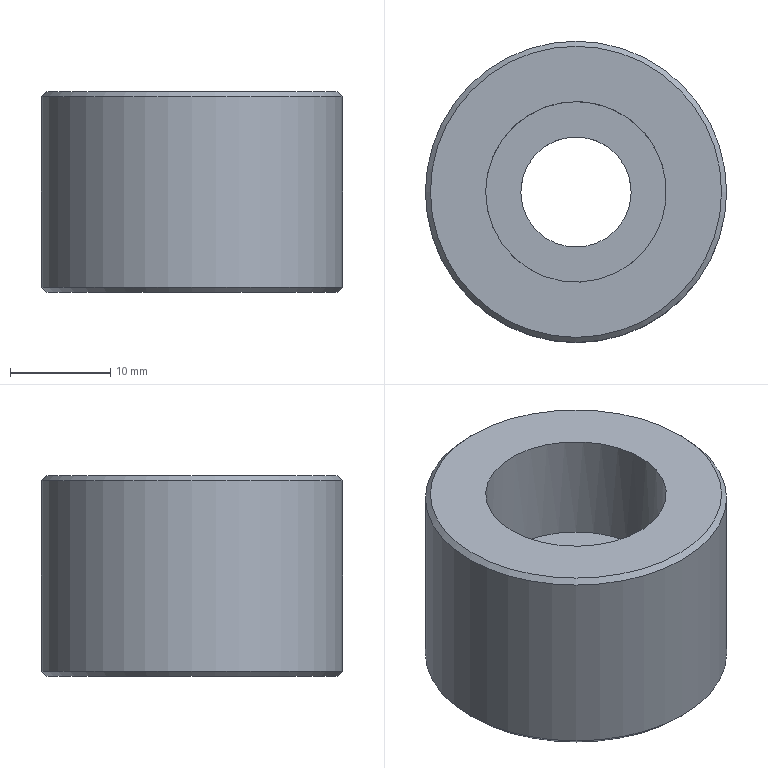Part | STEP file | solid 178 | 1 solid | 8 faces | box 30 x 30 x 20 mm | volume 10459 mm3 | plane 3 | cylinder 3 | cone 2 | commonest cylinder face diameters 11 x1 18 x1 30 x1